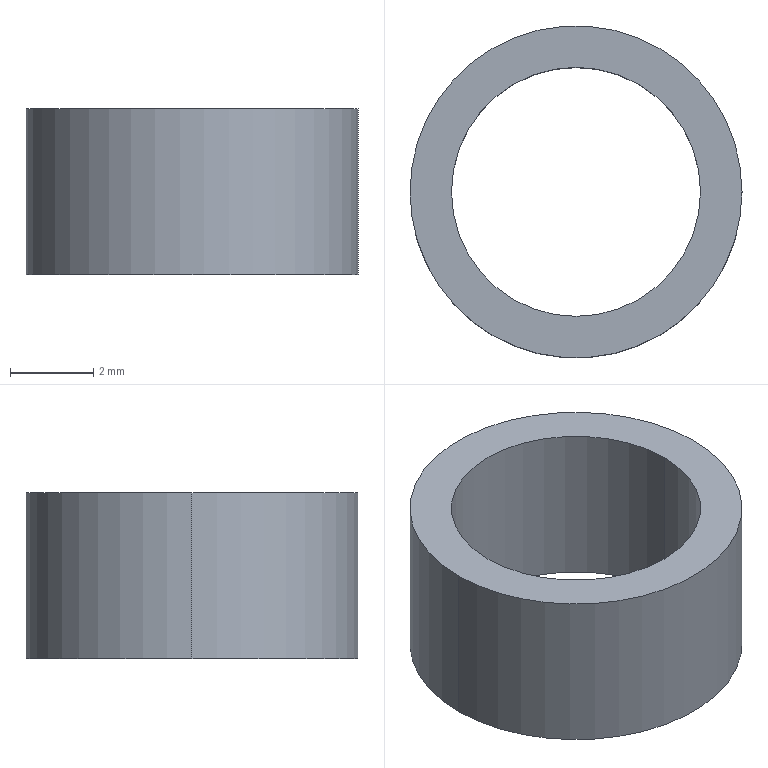Part | SolidWorks | features Extrusion 1 | 1 solid | 6 faces | box 8 x 8 x 4 mm | volume 87.965 mm3 | cylinder 4 | plane 2 | commonest cylinder face diameters 6 x2 8 x2
STEP:
#1=CARTESIAN_POINT('',(-3.,0.,4.));
#2=VERTEX_POINT('',#1);
#3=CARTESIAN_POINT('',(3.,0.,4.));
#4=VERTEX_POINT('',#3);
#5=CARTESIAN_POINT('',(0.,0.,4.));
#6=DIRECTION('',(0.,0.,1.));
#7=DIRECTION('',(1.,0.,0.));
#8=AXIS2_PLACEMENT_3D('',#5,#6,#7);
#9=CIRCLE('',#8,3.);
#10=EDGE_CURVE('',#2,#4,#9,.T.);
#11=ORIENTED_EDGE('',*,*,#10,.T.);
#12=CARTESIAN_POINT('',(3.,0.,0.));
#13=VERTEX_POINT('',#12);
#14=CARTESIAN_POINT('',(3.,0.,4.));
#15=DIRECTION('',(0.,0.,-1.));
#16=VECTOR('',#15,1000.);
#17=LINE('',#14,#16);
#18=EDGE_CURVE('',#4,#13,#17,.T.);
#19=ORIENTED_EDGE('',*,*,#18,.T.);
#20=CARTESIAN_POINT('',(-3.,0.,0.));
#21=VERTEX_POINT('',#20);
#22=CARTESIAN_POINT('',(0.,0.,0.));
#23=DIRECTION('',(0.,0.,1.));
#24=DIRECTION('',(1.,0.,0.));
#25=AXIS2_PLACEMENT_3D('',#22,#23,#24);
#26=CIRCLE('',#25,3.);
#27=EDGE_CURVE('',#21,#13,#26,.T.);
#28=ORIENTED_EDGE('',*,*,#27,.F.);
#29=CARTESIAN_POINT('',(-3.,0.,4.));
#30=DIRECTION('',(0.,0.,-1.));
#31=VECTOR('',#30,1000.);
#32=LINE('',#29,#31);
#33=EDGE_CURVE('',#2,#21,#32,.T.);
#34=ORIENTED_EDGE('',*,*,#33,.F.);
#35=EDGE_LOOP('',(#11,#19,#28,#34));
#36=FACE_OUTER_BOUND('',#35,.T.);
#37=CARTESIAN_POINT('',(0.,0.,4.));
#38=DIRECTION('',(0.,0.,-1.));
#39=DIRECTION('',(-1.,0.,0.));
#40=AXIS2_PLACEMENT_3D('',#37,#38,#39);
#41=CYLINDRICAL_SURFACE('',#40,3.);
#42=ADVANCED_FACE('',(#36),#41,.F.);
#43=CARTESIAN_POINT('',(4.,0.,4.));
#44=VERTEX_POINT('',#43);
#45=CARTESIAN_POINT('',(-4.,0.,4.));
#46=VERTEX_POINT('',#45);
#47=CARTESIAN_POINT('',(0.,0.,4.));
#48=DIRECTION('',(0.,0.,1.));
#49=DIRECTION('',(1.,0.,0.));
#50=AXIS2_PLACEMENT_3D('',#47,#48,#49);
#51=CIRCLE('',#50,4.);
#52=EDGE_CURVE('',#44,#46,#51,.T.);
#53=ORIENTED_EDGE('',*,*,#52,.F.);
#54=CARTESIAN_POINT('',(4.,0.,0.));
#55=VERTEX_POINT('',#54);
#56=CARTESIAN_POINT('',(4.,0.,4.));
#57=DIRECTION('',(0.,0.,-1.));
#58=VECTOR('',#57,1000.);
#59=LINE('',#56,#58);
#60=EDGE_CURVE('',#44,#55,#59,.T.);
#61=ORIENTED_EDGE('',*,*,#60,.T.);
#62=CARTESIAN_POINT('',(-4.,0.,0.));
#63=VERTEX_POINT('',#62);
#64=CARTESIAN_POINT('',(0.,0.,0.));
#65=DIRECTION('',(0.,0.,1.));
#66=DIRECTION('',(1.,0.,0.));
#67=AXIS2_PLACEMENT_3D('',#64,#65,#66);
#68=CIRCLE('',#67,4.);
#69=EDGE_CURVE('',#55,#63,#68,.T.);
#70=ORIENTED_EDGE('',*,*,#69,.T.);
#71=CARTESIAN_POINT('',(-4.,0.,4.));
#72=DIRECTION('',(0.,0.,-1.));
#73=VECTOR('',#72,1000.);
#74=LINE('',#71,#73);
#75=EDGE_CURVE('',#46,#63,#74,.T.);
#76=ORIENTED_EDGE('',*,*,#75,.F.);
#77=EDGE_LOOP('',(#53,#61,#70,#76));
#78=FACE_OUTER_BOUND('',#77,.T.);
#79=CARTESIAN_POINT('',(0.,0.,4.));
#80=DIRECTION('',(0.,0.,-1.));
#81=DIRECTION('',(-1.,0.,0.));
#82=AXIS2_PLACEMENT_3D('',#79,#80,#81);
#83=CYLINDRICAL_SURFACE('',#82,4.);
#84=ADVANCED_FACE('',(#78),#83,.T.);
#85=CARTESIAN_POINT('',(0.,0.,4.));
#86=DIRECTION('',(0.,0.,1.));
#87=DIRECTION('',(1.,0.,0.));
#88=AXIS2_PLACEMENT_3D('',#85,#86,#87);
#89=CIRCLE('',#88,4.);
#90=EDGE_CURVE('',#46,#44,#89,.T.);
#91=ORIENTED_EDGE('',*,*,#90,.T.);
#92=ORIENTED_EDGE('',*,*,#52,.T.);
#93=EDGE_LOOP('',(#91,#92));
#94=FACE_OUTER_BOUND('',#93,.T.);
#95=ORIENTED_EDGE('',*,*,#10,.F.);
#96=CARTESIAN_POINT('',(0.,0.,4.));
#97=DIRECTION('',(0.,0.,1.));
#98=DIRECTION('',(1.,0.,0.));
#99=AXIS2_PLACEMENT_3D('',#96,#97,#98);
#100=CIRCLE('',#99,3.);
#101=EDGE_CURVE('',#4,#2,#100,.T.);
#102=ORIENTED_EDGE('',*,*,#101,.F.);
#103=EDGE_LOOP('',(#95,#102));
#104=FACE_BOUND('',#103,.T.);
#105=CARTESIAN_POINT('',(0.,0.,4.));
#106=DIRECTION('',(0.,0.,1.));
#107=DIRECTION('',(1.,0.,0.));
#108=AXIS2_PLACEMENT_3D('',#105,#106,#107);
#109=PLANE('',#108);
#110=ADVANCED_FACE('',(#94,#104),#109,.T.);
#111=CARTESIAN_POINT('',(0.,0.,0.));
#112=DIRECTION('',(0.,0.,1.));
#113=DIRECTION('',(1.,0.,0.));
#114=AXIS2_PLACEMENT_3D('',#111,#112,#113);
#115=CIRCLE('',#114,4.);
#116=EDGE_CURVE('',#63,#55,#115,.T.);
#117=ORIENTED_EDGE('',*,*,#116,.F.);
#118=ORIENTED_EDGE('',*,*,#69,.F.);
#119=EDGE_LOOP('',(#117,#118));
#120=FACE_OUTER_BOUND('',#119,.T.);
#121=ORIENTED_EDGE('',*,*,#27,.T.);
#122=CARTESIAN_POINT('',(0.,0.,0.));
#123=DIRECTION('',(0.,0.,1.));
#124=DIRECTION('',(1.,0.,0.));
#125=AXIS2_PLACEMENT_3D('',#122,#123,#124);
#126=CIRCLE('',#125,3.);
#127=EDGE_CURVE('',#13,#21,#126,.T.);
#128=ORIENTED_EDGE('',*,*,#127,.T.);
#129=EDGE_LOOP('',(#121,#128));
#130=FACE_BOUND('',#129,.T.);
#131=CARTESIAN_POINT('',(0.,0.,0.));
#132=DIRECTION('',(0.,0.,1.));
#133=DIRECTION('',(1.,0.,0.));
#134=AXIS2_PLACEMENT_3D('',#131,#132,#133);
#135=PLANE('',#134);
#136=ADVANCED_FACE('',(#120,#130),#135,.F.);
#137=ORIENTED_EDGE('',*,*,#60,.F.);
#138=ORIENTED_EDGE('',*,*,#90,.F.);
#139=ORIENTED_EDGE('',*,*,#75,.T.);
#140=ORIENTED_EDGE('',*,*,#116,.T.);
#141=EDGE_LOOP('',(#137,#138,#139,#140));
#142=FACE_OUTER_BOUND('',#141,.T.);
#143=CARTESIAN_POINT('',(0.,0.,4.));
#144=DIRECTION('',(0.,0.,-1.));
#145=DIRECTION('',(-1.,0.,0.));
#146=AXIS2_PLACEMENT_3D('',#143,#144,#145);
#147=CYLINDRICAL_SURFACE('',#146,4.);
#148=ADVANCED_FACE('',(#142),#147,.T.);
#149=ORIENTED_EDGE('',*,*,#18,.F.);
#150=ORIENTED_EDGE('',*,*,#101,.T.);
#151=ORIENTED_EDGE('',*,*,#33,.T.);
#152=ORIENTED_EDGE('',*,*,#127,.F.);
#153=EDGE_LOOP('',(#149,#150,#151,#152));
#154=FACE_OUTER_BOUND('',#153,.T.);
#155=CARTESIAN_POINT('',(0.,0.,4.));
#156=DIRECTION('',(0.,0.,-1.));
#157=DIRECTION('',(-1.,0.,0.));
#158=AXIS2_PLACEMENT_3D('',#155,#156,#157);
#159=CYLINDRICAL_SURFACE('',#158,3.);
#160=ADVANCED_FACE('',(#154),#159,.F.);
#161=CLOSED_SHELL('',(#42,#84,#110,#136,#148,#160));
#162=MANIFOLD_SOLID_BREP('',#161);
#163=CARTESIAN_POINT('',(0.,0.,0.));
#164=DIRECTION('',(0.,0.,1.));
#165=DIRECTION('',(1.,0.,0.));
#166=AXIS2_PLACEMENT_3D('',#163,#164,#165);
#167=(LENGTH_UNIT()NAMED_UNIT(*)SI_UNIT(.MILLI.,.METRE.));
#168=UNCERTAINTY_MEASURE_WITH_UNIT(LENGTH_MEASURE(0.00001),#167,'','');
#169=(NAMED_UNIT(*)PLANE_ANGLE_UNIT()SI_UNIT($,.RADIAN.));
#170=(NAMED_UNIT(*)SI_UNIT($,.STERADIAN.)SOLID_ANGLE_UNIT());
#171=(GEOMETRIC_REPRESENTATION_CONTEXT(3)GLOBAL_UNCERTAINTY_ASSIGNED_CONTEXT((#168))GLOBAL_UNIT_ASSIGNED_CONTEXT((#167,#169,#170))REPRESENTATION_CONTEXT('',''));
#172=ADVANCED_BREP_SHAPE_REPRESENTATION('',(#162,#166),#171);